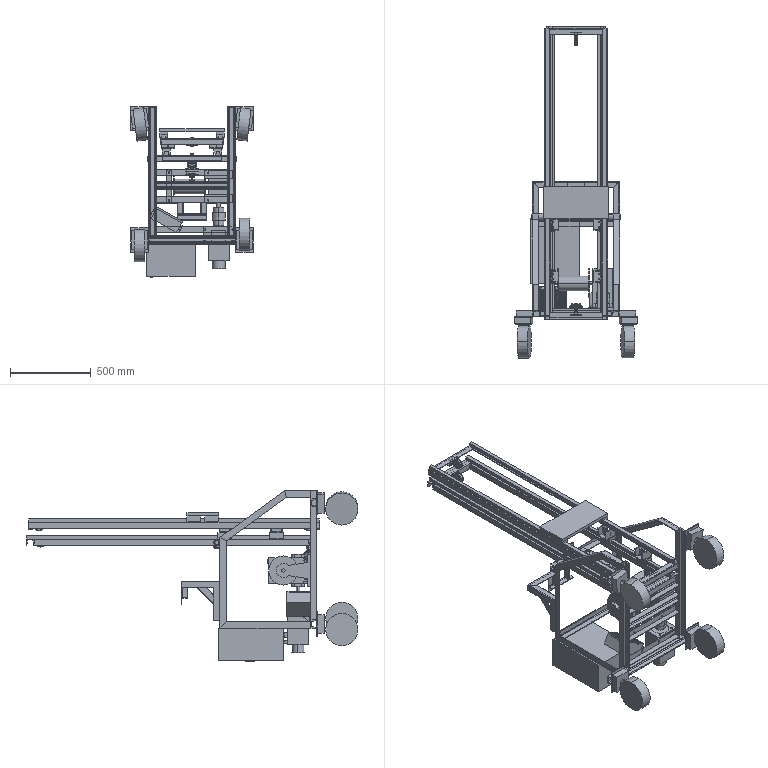Part | SolidWorks | 94 solids | 1894 faces | box 763.29 x 2055 x 1056 mm | volume 63128223 mm3 | plane 1027 | cylinder 766 | cone 96 | torus 4 | spline 1 | commonest cylinder face diameters 6.5 x284 5 x98 10 x50 2.667 x44 7 x44 4 x37